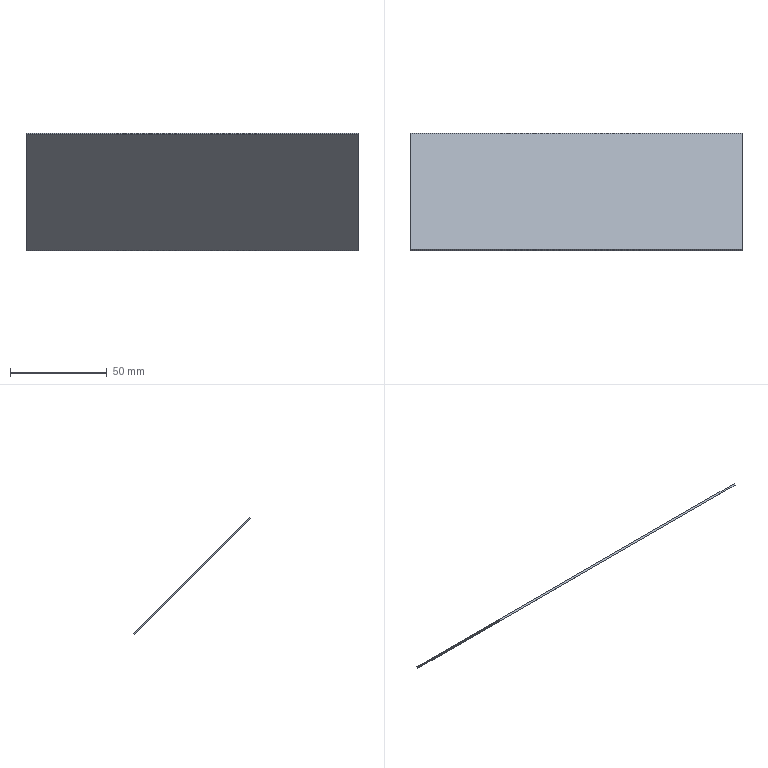Part | SolidWorks | features BaseBody 1 | 1 solid | 6 faces | box 172 x 61 x 61 mm | volume 14666 mm3 | plane 6
STEP:
#1=CARTESIAN_POINT('',(-86.,-29.586,62.));
#2=VERTEX_POINT('',#1);
#3=CARTESIAN_POINT('',(-86.,-30.293,61.293));
#4=VERTEX_POINT('',#3);
#5=CARTESIAN_POINT('',(-86.,-29.939,61.646));
#6=DIRECTION('',(0.,-0.7071,-0.7071));
#7=VECTOR('',#6,1000.);
#8=LINE('',#5,#7);
#9=EDGE_CURVE('',#2,#4,#8,.T.);
#10=ORIENTED_EDGE('',*,*,#9,.F.);
#11=CARTESIAN_POINT('',(-86.,30.707,1.707));
#12=VERTEX_POINT('',#11);
#13=CARTESIAN_POINT('',(-86.,31.913,0.5012));
#14=DIRECTION('',(0.,-0.7071,0.7071));
#15=VECTOR('',#14,1000.);
#16=LINE('',#13,#15);
#17=EDGE_CURVE('',#12,#2,#16,.T.);
#18=ORIENTED_EDGE('',*,*,#17,.F.);
#19=CARTESIAN_POINT('',(-86.,30.,1.));
#20=VERTEX_POINT('',#19);
#21=CARTESIAN_POINT('',(-86.,30.354,1.354));
#22=DIRECTION('',(0.,0.7071,0.7071));
#23=VECTOR('',#22,1000.);
#24=LINE('',#21,#23);
#25=EDGE_CURVE('',#20,#12,#24,.T.);
#26=ORIENTED_EDGE('',*,*,#25,.F.);
#27=CARTESIAN_POINT('',(-86.,-31.499,62.499));
#28=DIRECTION('',(0.,0.7071,-0.7071));
#29=VECTOR('',#28,1000.);
#30=LINE('',#27,#29);
#31=EDGE_CURVE('',#4,#20,#30,.T.);
#32=ORIENTED_EDGE('',*,*,#31,.F.);
#33=EDGE_LOOP('',(#10,#18,#26,#32));
#34=FACE_OUTER_BOUND('',#33,.T.);
#35=CARTESIAN_POINT('',(-86.,31.927,63.22));
#36=DIRECTION('',(1.,0.,0.));
#37=DIRECTION('',(0.,-1.,0.));
#38=AXIS2_PLACEMENT_3D('',#35,#36,#37);
#39=PLANE('',#38);
#40=ADVANCED_FACE('',(#34),#39,.F.);
#41=CARTESIAN_POINT('',(86.,30.,1.));
#42=VERTEX_POINT('',#41);
#43=CARTESIAN_POINT('',(86.,-30.293,61.293));
#44=VERTEX_POINT('',#43);
#45=CARTESIAN_POINT('',(86.,-0.1464,31.146));
#46=DIRECTION('',(0.,-0.7071,0.7071));
#47=VECTOR('',#46,1000.);
#48=LINE('',#45,#47);
#49=EDGE_CURVE('',#42,#44,#48,.T.);
#50=ORIENTED_EDGE('',*,*,#49,.T.);
#51=CARTESIAN_POINT('',(0.,-30.293,61.293));
#52=DIRECTION('',(-1.,0.,0.));
#53=VECTOR('',#52,1000.);
#54=LINE('',#51,#53);
#55=EDGE_CURVE('',#44,#4,#54,.T.);
#56=ORIENTED_EDGE('',*,*,#55,.T.);
#57=ORIENTED_EDGE('',*,*,#31,.T.);
#58=CARTESIAN_POINT('',(0.,30.,1.));
#59=DIRECTION('',(1.,0.,0.));
#60=VECTOR('',#59,1000.);
#61=LINE('',#58,#60);
#62=EDGE_CURVE('',#20,#42,#61,.T.);
#63=ORIENTED_EDGE('',*,*,#62,.T.);
#64=EDGE_LOOP('',(#50,#56,#57,#63));
#65=FACE_OUTER_BOUND('',#64,.T.);
#66=CARTESIAN_POINT('',(-89.44,-31.499,62.499));
#67=DIRECTION('',(0.,-0.7071,-0.7071));
#68=DIRECTION('',(0.,0.7071,-0.7071));
#69=AXIS2_PLACEMENT_3D('',#66,#67,#68);
#70=PLANE('',#69);
#71=ADVANCED_FACE('',(#65),#70,.T.);
#72=CARTESIAN_POINT('',(86.,-29.586,62.));
#73=VERTEX_POINT('',#72);
#74=CARTESIAN_POINT('',(86.,30.707,1.707));
#75=VERTEX_POINT('',#74);
#76=CARTESIAN_POINT('',(86.,0.5607,31.854));
#77=DIRECTION('',(0.,0.7071,-0.7071));
#78=VECTOR('',#77,1000.);
#79=LINE('',#76,#78);
#80=EDGE_CURVE('',#73,#75,#79,.T.);
#81=ORIENTED_EDGE('',*,*,#80,.T.);
#82=CARTESIAN_POINT('',(0.,30.707,1.707));
#83=DIRECTION('',(-1.,0.,0.));
#84=VECTOR('',#83,1000.);
#85=LINE('',#82,#84);
#86=EDGE_CURVE('',#75,#12,#85,.T.);
#87=ORIENTED_EDGE('',*,*,#86,.T.);
#88=ORIENTED_EDGE('',*,*,#17,.T.);
#89=CARTESIAN_POINT('',(0.,-29.586,62.));
#90=DIRECTION('',(1.,0.,0.));
#91=VECTOR('',#90,1000.);
#92=LINE('',#89,#91);
#93=EDGE_CURVE('',#2,#73,#92,.T.);
#94=ORIENTED_EDGE('',*,*,#93,.T.);
#95=EDGE_LOOP('',(#81,#87,#88,#94));
#96=FACE_OUTER_BOUND('',#95,.T.);
#97=CARTESIAN_POINT('',(-89.44,31.913,0.5012));
#98=DIRECTION('',(0.,0.7071,0.7071));
#99=DIRECTION('',(0.,-0.7071,0.7071));
#100=AXIS2_PLACEMENT_3D('',#97,#98,#99);
#101=PLANE('',#100);
#102=ADVANCED_FACE('',(#96),#101,.T.);
#103=CARTESIAN_POINT('',(86.,-29.939,61.646));
#104=DIRECTION('',(0.,0.7071,0.7071));
#105=VECTOR('',#104,1000.);
#106=LINE('',#103,#105);
#107=EDGE_CURVE('',#44,#73,#106,.T.);
#108=ORIENTED_EDGE('',*,*,#107,.T.);
#109=ORIENTED_EDGE('',*,*,#93,.F.);
#110=ORIENTED_EDGE('',*,*,#9,.T.);
#111=ORIENTED_EDGE('',*,*,#55,.F.);
#112=EDGE_LOOP('',(#108,#109,#110,#111));
#113=FACE_OUTER_BOUND('',#112,.T.);
#114=CARTESIAN_POINT('',(-89.44,-29.423,62.163));
#115=DIRECTION('',(0.,-0.7071,0.7071));
#116=DIRECTION('',(0.,-0.7071,-0.7071));
#117=AXIS2_PLACEMENT_3D('',#114,#115,#116);
#118=PLANE('',#117);
#119=ADVANCED_FACE('',(#113),#118,.T.);
#120=ORIENTED_EDGE('',*,*,#107,.F.);
#121=ORIENTED_EDGE('',*,*,#49,.F.);
#122=CARTESIAN_POINT('',(86.,29.837,0.8367));
#123=DIRECTION('',(0.,-0.7071,-0.7071));
#124=VECTOR('',#123,1000.);
#125=LINE('',#122,#124);
#126=EDGE_CURVE('',#75,#42,#125,.T.);
#127=ORIENTED_EDGE('',*,*,#126,.F.);
#128=ORIENTED_EDGE('',*,*,#80,.F.);
#129=EDGE_LOOP('',(#120,#121,#127,#128));
#130=FACE_OUTER_BOUND('',#129,.T.);
#131=CARTESIAN_POINT('',(86.,31.927,-0.22));
#132=DIRECTION('',(-1.,0.,0.));
#133=DIRECTION('',(0.,-1.,0.));
#134=AXIS2_PLACEMENT_3D('',#131,#132,#133);
#135=PLANE('',#134);
#136=ADVANCED_FACE('',(#130),#135,.F.);
#137=ORIENTED_EDGE('',*,*,#126,.T.);
#138=ORIENTED_EDGE('',*,*,#62,.F.);
#139=ORIENTED_EDGE('',*,*,#25,.T.);
#140=ORIENTED_EDGE('',*,*,#86,.F.);
#141=EDGE_LOOP('',(#137,#138,#139,#140));
#142=FACE_OUTER_BOUND('',#141,.T.);
#143=CARTESIAN_POINT('',(-89.44,29.837,0.8367));
#144=DIRECTION('',(0.,0.7071,-0.7071));
#145=DIRECTION('',(0.,0.7071,0.7071));
#146=AXIS2_PLACEMENT_3D('',#143,#144,#145);
#147=PLANE('',#146);
#148=ADVANCED_FACE('',(#142),#147,.T.);
#149=CLOSED_SHELL('',(#40,#71,#102,#119,#136,#148));
#150=MANIFOLD_SOLID_BREP('',#149);
#151=CARTESIAN_POINT('',(0.,0.,0.));
#152=DIRECTION('',(0.,0.,1.));
#153=DIRECTION('',(1.,0.,0.));
#154=AXIS2_PLACEMENT_3D('',#151,#152,#153);
#155=(LENGTH_UNIT()NAMED_UNIT(*)SI_UNIT(.MILLI.,.METRE.));
#156=UNCERTAINTY_MEASURE_WITH_UNIT(LENGTH_MEASURE(0.00001),#155,'','');
#157=(NAMED_UNIT(*)PLANE_ANGLE_UNIT()SI_UNIT($,.RADIAN.));
#158=(NAMED_UNIT(*)SI_UNIT($,.STERADIAN.)SOLID_ANGLE_UNIT());
#159=(GEOMETRIC_REPRESENTATION_CONTEXT(3)GLOBAL_UNCERTAINTY_ASSIGNED_CONTEXT((#156))GLOBAL_UNIT_ASSIGNED_CONTEXT((#155,#157,#158))REPRESENTATION_CONTEXT('',''));
#160=ADVANCED_BREP_SHAPE_REPRESENTATION('',(#150,#154),#159);